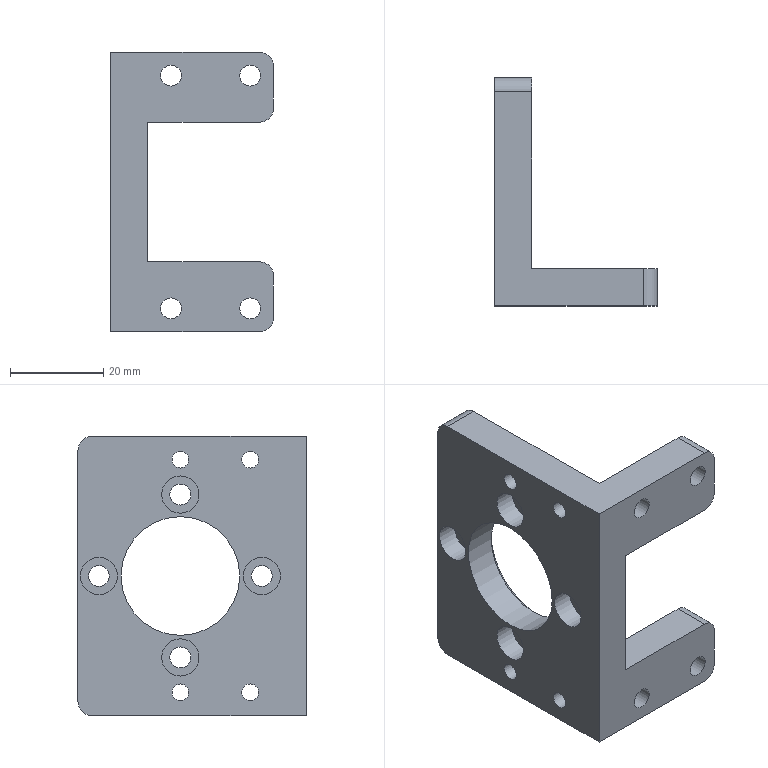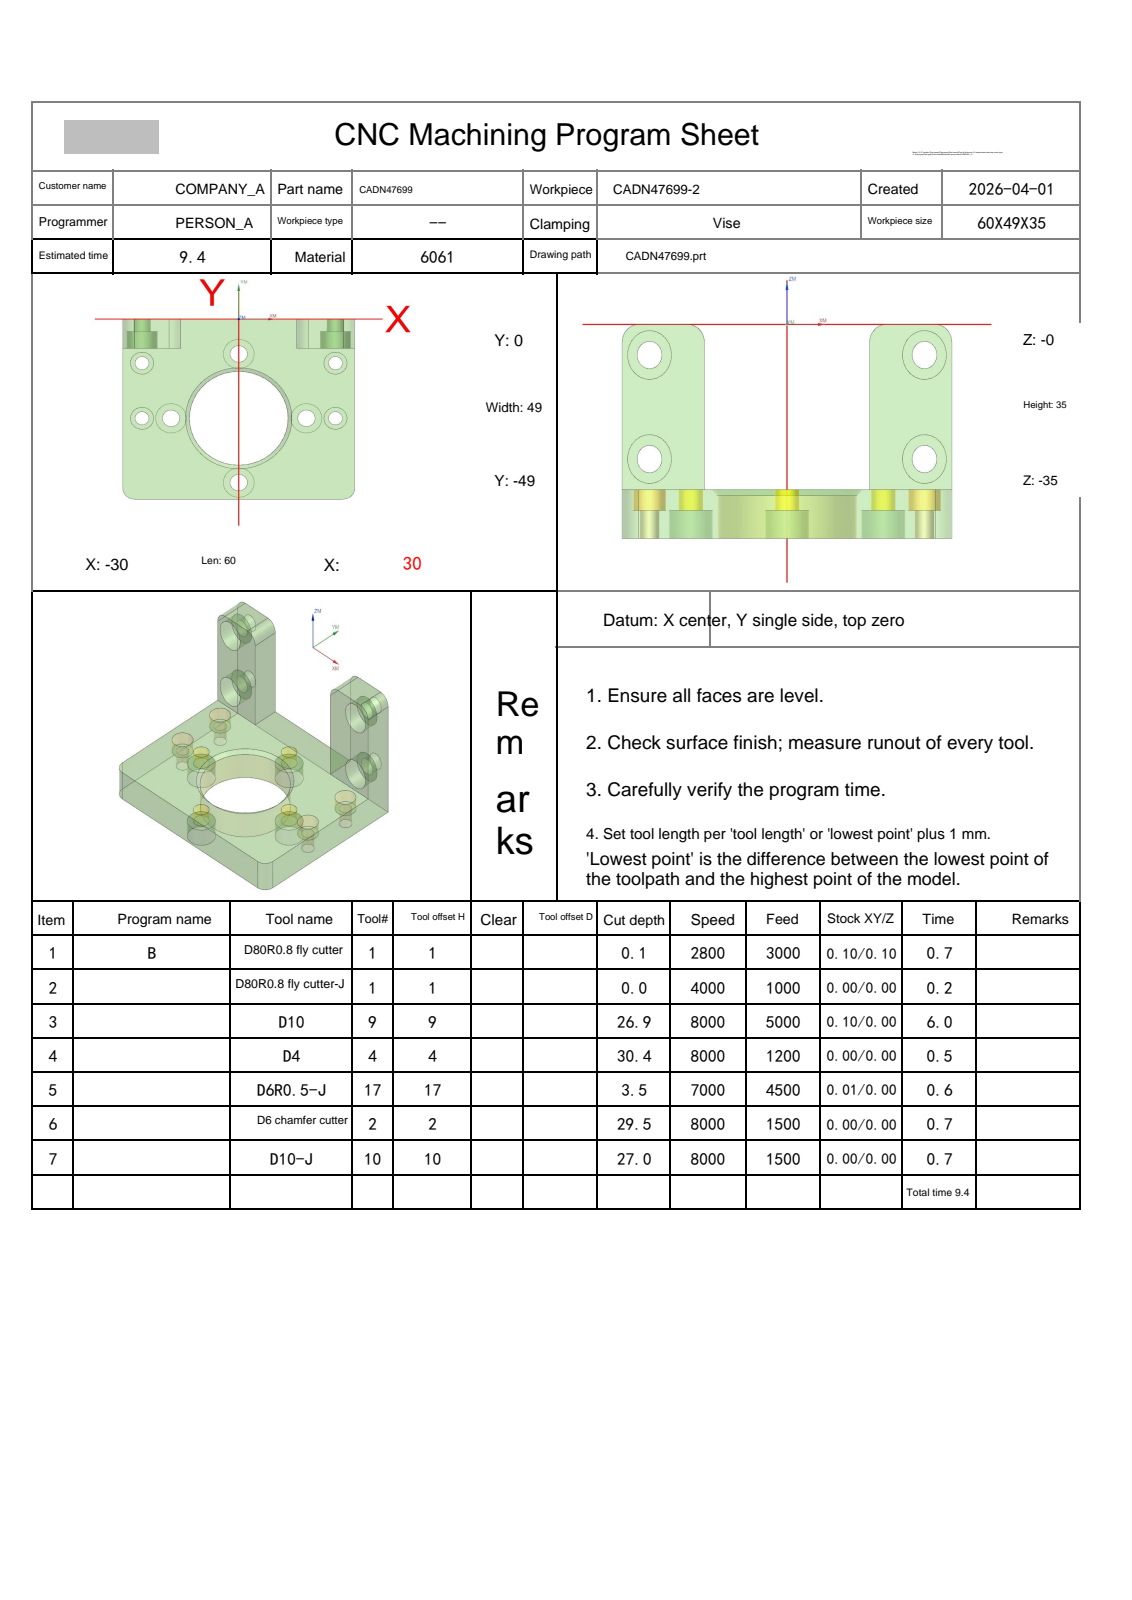NC program | NX | posted by the shop | part box 35 x 49 x 60 mm
Lines 1 to 110 of 5920:
%
O0001
(Machine time: 10.53 MIN)
(===Total Tool:6===)
(T1=D80R0.8 fly cutter D=80.  R=0.8  D-  H01 Z=0.    )
(T9=D10     D=10.  R=0.   D-  H09 Z=-26.9 )
(T4=D4      D=4.   R=0.   D-  H04 Z=-30.4 )
(T17=D6R0.5-J D=6.   R=0.5  D-  H17 Z=-3.5  )
(T2=D6 chamfer cutter   D=6.   R=0.   D-  H02 Z=-29.55)
(T10=D10-J  D=10.  R=0.   D10 H10 Z=-27.  )
G80 G90 G17 G49 G40
G91 G28 Z0
M01
N1 T01 M06
(D80R0.8 fly cutter  D=80. R=0.8 H=01 ce=0.10 di=0.10)
G00 G90 G54 X82.097 Y-24.5 M03 S2800
G43 H01 Z20.
M08
Z6.011
G01 Z4.011 F3000.
X70.097
X-70.097
X-82.097
Z6.011
G00 X82.097
Z5.522
G01 Z3.522
X70.097
X-70.097
X-82.097
Z5.522
G00 X82.097
Z5.033
G01 Z3.033
X70.097
X-70.097
X-82.097
Z5.033
G00 X82.097
Z4.544
G01 Z2.544
X70.097
X-70.097
X-82.097
Z4.544
G00 Z20.
X82.097
Z4.056
G01 Z2.056
X70.097
X-70.097
X-82.097
Z4.056
G00 Z20.
X82.097
Z3.567
G01 Z1.567
X70.097
X-70.097
X-82.097
Z3.567
G00 Z20.
X82.097
Z3.078
G01 Z1.078
X70.097
X-70.097
X-82.097
Z3.078
G00 Z20.
X82.097
Z2.589
G01 Z.589
X70.097
X-70.097
X-82.097
Z2.589
G00 Z20.
X82.097
Z2.1
G01 Z.1
X70.097
X-70.097
X-82.097
Z2.1
G00 Z20.
G91 G28 Z0.0
M05
M09
G91 G28 Z0.0
M01
N2 T01 M06
(D80R0.8 fly cutter-J  D=80. R=0.8 H=01 ce=0.00 di=0.00)
G00 G90 G54 X81.999 Y-24.49 M03 S4000
G43 H01 Z20.
M08
Z2.
G01 Z0.0 F1000.
X69.999 Y-24.491
X-69.999 Y-24.508
X-81.999 Y-24.51
Z2.
G00 Z20.
G91 G28 Z0.0
M05
M09
G91 G28 Z0.0
M01